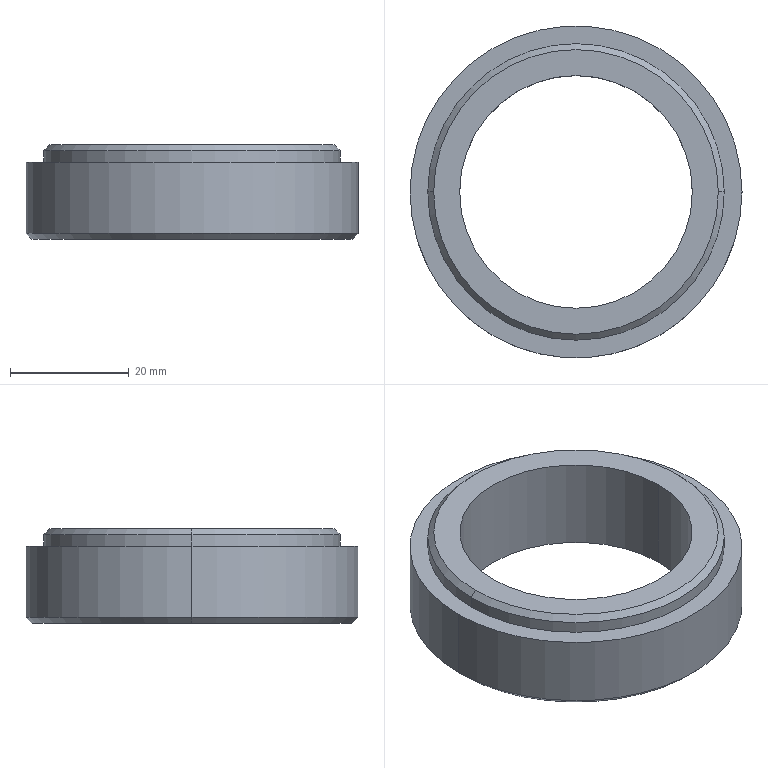Part | SolidWorks | features 3DProfileFeature 1, Chamfer 1, Extrusion 1, HoleWzd 1, ICE 1 | 1 solid | 13 faces | box 56 x 56 x 16 mm | volume 18386 mm3 | cylinder 6 | cone 4 | plane 3 | commonest cylinder face diameters 39.25 x2 50 x2 56 x2
STEP:
#1=CARTESIAN_POINT('',(-19.625,0.,0.));
#2=VERTEX_POINT('',#1);
#3=CARTESIAN_POINT('',(19.625,0.,0.));
#4=VERTEX_POINT('',#3);
#5=CARTESIAN_POINT('',(0.,0.,0.));
#6=DIRECTION('',(0.,0.,1.));
#7=DIRECTION('',(1.,0.,0.));
#8=AXIS2_PLACEMENT_3D('',#5,#6,#7);
#9=CIRCLE('',#8,19.625);
#10=EDGE_CURVE('',#2,#4,#9,.T.);
#11=ORIENTED_EDGE('',*,*,#10,.F.);
#12=CARTESIAN_POINT('',(-19.625,0.,16.));
#13=VERTEX_POINT('',#12);
#14=CARTESIAN_POINT('',(-19.625,0.,16.));
#15=DIRECTION('',(0.,0.,1.));
#16=VECTOR('',#15,1000.);
#17=LINE('',#14,#16);
#18=EDGE_CURVE('',#2,#13,#17,.T.);
#19=ORIENTED_EDGE('',*,*,#18,.T.);
#20=CARTESIAN_POINT('',(19.625,0.,16.));
#21=VERTEX_POINT('',#20);
#22=CARTESIAN_POINT('',(0.,0.,16.));
#23=DIRECTION('',(0.,0.,1.));
#24=DIRECTION('',(1.,0.,0.));
#25=AXIS2_PLACEMENT_3D('',#22,#23,#24);
#26=CIRCLE('',#25,19.625);
#27=EDGE_CURVE('',#13,#21,#26,.T.);
#28=ORIENTED_EDGE('',*,*,#27,.T.);
#29=CARTESIAN_POINT('',(19.625,0.,16.));
#30=DIRECTION('',(0.,0.,1.));
#31=VECTOR('',#30,1000.);
#32=LINE('',#29,#31);
#33=EDGE_CURVE('',#4,#21,#32,.T.);
#34=ORIENTED_EDGE('',*,*,#33,.F.);
#35=EDGE_LOOP('',(#11,#19,#28,#34));
#36=FACE_OUTER_BOUND('',#35,.T.);
#37=CARTESIAN_POINT('',(0.,0.,16.));
#38=DIRECTION('',(0.,0.,1.));
#39=DIRECTION('',(1.,0.,0.));
#40=AXIS2_PLACEMENT_3D('',#37,#38,#39);
#41=CYLINDRICAL_SURFACE('',#40,19.625);
#42=ADVANCED_FACE('',(#36),#41,.F.);
#43=CARTESIAN_POINT('',(24.,0.,16.));
#44=VERTEX_POINT('',#43);
#45=CARTESIAN_POINT('',(-24.,0.,16.));
#46=VERTEX_POINT('',#45);
#47=CARTESIAN_POINT('',(0.,0.,16.));
#48=DIRECTION('',(0.,0.,1.));
#49=DIRECTION('',(1.,0.,0.));
#50=AXIS2_PLACEMENT_3D('',#47,#48,#49);
#51=CIRCLE('',#50,24.);
#52=EDGE_CURVE('',#44,#46,#51,.T.);
#53=ORIENTED_EDGE('',*,*,#52,.F.);
#54=CARTESIAN_POINT('',(25.,0.,15.));
#55=VERTEX_POINT('',#54);
#56=CARTESIAN_POINT('',(24.,0.,16.));
#57=DIRECTION('',(0.7071,0.,-0.7071));
#58=VECTOR('',#57,1000.);
#59=LINE('',#56,#58);
#60=EDGE_CURVE('',#44,#55,#59,.T.);
#61=ORIENTED_EDGE('',*,*,#60,.T.);
#62=CARTESIAN_POINT('',(-25.,0.,15.));
#63=VERTEX_POINT('',#62);
#64=CARTESIAN_POINT('',(0.,0.,15.));
#65=DIRECTION('',(0.,0.,-1.));
#66=DIRECTION('',(1.,0.,0.));
#67=AXIS2_PLACEMENT_3D('',#64,#65,#66);
#68=CIRCLE('',#67,25.);
#69=EDGE_CURVE('',#63,#55,#68,.T.);
#70=ORIENTED_EDGE('',*,*,#69,.F.);
#71=CARTESIAN_POINT('',(-24.,0.,16.));
#72=DIRECTION('',(-0.7071,0.,-0.7071));
#73=VECTOR('',#72,1000.);
#74=LINE('',#71,#73);
#75=EDGE_CURVE('',#46,#63,#74,.T.);
#76=ORIENTED_EDGE('',*,*,#75,.F.);
#77=EDGE_LOOP('',(#53,#61,#70,#76));
#78=FACE_OUTER_BOUND('',#77,.T.);
#79=CARTESIAN_POINT('',(0.,0.,16.));
#80=DIRECTION('',(0.,0.,-1.));
#81=DIRECTION('',(-1.,0.,0.));
#82=AXIS2_PLACEMENT_3D('',#79,#80,#81);
#83=CONICAL_SURFACE('',#82,24.,0.7854);
#84=ADVANCED_FACE('',(#78),#83,.T.);
#85=CARTESIAN_POINT('',(-27.,0.,0.));
#86=VERTEX_POINT('',#85);
#87=CARTESIAN_POINT('',(27.,0.,0.));
#88=VERTEX_POINT('',#87);
#89=CARTESIAN_POINT('',(0.,0.,0.));
#90=DIRECTION('',(0.,0.,-1.));
#91=DIRECTION('',(1.,0.,0.));
#92=AXIS2_PLACEMENT_3D('',#89,#90,#91);
#93=CIRCLE('',#92,27.);
#94=EDGE_CURVE('',#86,#88,#93,.T.);
#95=ORIENTED_EDGE('',*,*,#94,.F.);
#96=CARTESIAN_POINT('',(-28.,0.,1.));
#97=VERTEX_POINT('',#96);
#98=CARTESIAN_POINT('',(-28.,0.,1.));
#99=DIRECTION('',(-0.7071,0.,0.7071));
#100=VECTOR('',#99,1000.);
#101=LINE('',#98,#100);
#102=EDGE_CURVE('',#86,#97,#101,.T.);
#103=ORIENTED_EDGE('',*,*,#102,.T.);
#104=CARTESIAN_POINT('',(28.,0.,1.));
#105=VERTEX_POINT('',#104);
#106=CARTESIAN_POINT('',(0.,0.,1.));
#107=DIRECTION('',(0.,0.,1.));
#108=DIRECTION('',(1.,0.,0.));
#109=AXIS2_PLACEMENT_3D('',#106,#107,#108);
#110=CIRCLE('',#109,28.);
#111=EDGE_CURVE('',#105,#97,#110,.T.);
#112=ORIENTED_EDGE('',*,*,#111,.F.);
#113=CARTESIAN_POINT('',(28.,0.,1.));
#114=DIRECTION('',(0.7071,0.,0.7071));
#115=VECTOR('',#114,1000.);
#116=LINE('',#113,#115);
#117=EDGE_CURVE('',#88,#105,#116,.T.);
#118=ORIENTED_EDGE('',*,*,#117,.F.);
#119=EDGE_LOOP('',(#95,#103,#112,#118));
#120=FACE_OUTER_BOUND('',#119,.T.);
#121=CARTESIAN_POINT('',(0.,0.,1.));
#122=DIRECTION('',(0.,0.,1.));
#123=DIRECTION('',(1.,0.,0.));
#124=AXIS2_PLACEMENT_3D('',#121,#122,#123);
#125=CONICAL_SURFACE('',#124,28.,0.7854);
#126=ADVANCED_FACE('',(#120),#125,.T.);
#127=ORIENTED_EDGE('',*,*,#69,.T.);
#128=CARTESIAN_POINT('',(25.,0.,13.));
#129=VERTEX_POINT('',#128);
#130=CARTESIAN_POINT('',(25.,0.,16.));
#131=DIRECTION('',(0.,0.,-1.));
#132=VECTOR('',#131,1000.);
#133=LINE('',#130,#132);
#134=EDGE_CURVE('',#55,#129,#133,.T.);
#135=ORIENTED_EDGE('',*,*,#134,.T.);
#136=CARTESIAN_POINT('',(-25.,0.,13.));
#137=VERTEX_POINT('',#136);
#138=CARTESIAN_POINT('',(0.,0.,13.));
#139=DIRECTION('',(0.,0.,1.));
#140=DIRECTION('',(1.,0.,0.));
#141=AXIS2_PLACEMENT_3D('',#138,#139,#140);
#142=CIRCLE('',#141,25.);
#143=EDGE_CURVE('',#129,#137,#142,.T.);
#144=ORIENTED_EDGE('',*,*,#143,.T.);
#145=CARTESIAN_POINT('',(-25.,0.,16.));
#146=DIRECTION('',(0.,0.,-1.));
#147=VECTOR('',#146,1000.);
#148=LINE('',#145,#147);
#149=EDGE_CURVE('',#63,#137,#148,.T.);
#150=ORIENTED_EDGE('',*,*,#149,.F.);
#151=EDGE_LOOP('',(#127,#135,#144,#150));
#152=FACE_OUTER_BOUND('',#151,.T.);
#153=CARTESIAN_POINT('',(0.,0.,16.));
#154=DIRECTION('',(0.,0.,-1.));
#155=DIRECTION('',(-1.,0.,0.));
#156=AXIS2_PLACEMENT_3D('',#153,#154,#155);
#157=CYLINDRICAL_SURFACE('',#156,25.);
#158=ADVANCED_FACE('',(#152),#157,.T.);
#159=CARTESIAN_POINT('',(28.,0.,13.));
#160=VERTEX_POINT('',#159);
#161=CARTESIAN_POINT('',(-28.,0.,13.));
#162=VERTEX_POINT('',#161);
#163=CARTESIAN_POINT('',(0.,0.,13.));
#164=DIRECTION('',(0.,0.,1.));
#165=DIRECTION('',(1.,0.,0.));
#166=AXIS2_PLACEMENT_3D('',#163,#164,#165);
#167=CIRCLE('',#166,28.);
#168=EDGE_CURVE('',#160,#162,#167,.T.);
#169=ORIENTED_EDGE('',*,*,#168,.F.);
#170=CARTESIAN_POINT('',(28.,0.,13.));
#171=DIRECTION('',(0.,0.,-1.));
#172=VECTOR('',#171,1000.);
#173=LINE('',#170,#172);
#174=EDGE_CURVE('',#160,#105,#173,.T.);
#175=ORIENTED_EDGE('',*,*,#174,.T.);
#176=ORIENTED_EDGE('',*,*,#111,.T.);
#177=CARTESIAN_POINT('',(-28.,0.,13.));
#178=DIRECTION('',(0.,0.,-1.));
#179=VECTOR('',#178,1000.);
#180=LINE('',#177,#179);
#181=EDGE_CURVE('',#162,#97,#180,.T.);
#182=ORIENTED_EDGE('',*,*,#181,.F.);
#183=EDGE_LOOP('',(#169,#175,#176,#182));
#184=FACE_OUTER_BOUND('',#183,.T.);
#185=CARTESIAN_POINT('',(0.,0.,13.));
#186=DIRECTION('',(0.,0.,-1.));
#187=DIRECTION('',(-1.,0.,0.));
#188=AXIS2_PLACEMENT_3D('',#185,#186,#187);
#189=CYLINDRICAL_SURFACE('',#188,28.);
#190=ADVANCED_FACE('',(#184),#189,.T.);
#191=CARTESIAN_POINT('',(0.,0.,13.));
#192=DIRECTION('',(0.,0.,1.));
#193=DIRECTION('',(1.,0.,0.));
#194=AXIS2_PLACEMENT_3D('',#191,#192,#193);
#195=CIRCLE('',#194,28.);
#196=EDGE_CURVE('',#162,#160,#195,.T.);
#197=ORIENTED_EDGE('',*,*,#196,.T.);
#198=ORIENTED_EDGE('',*,*,#168,.T.);
#199=EDGE_LOOP('',(#197,#198));
#200=FACE_OUTER_BOUND('',#199,.T.);
#201=CARTESIAN_POINT('',(0.,0.,13.));
#202=DIRECTION('',(0.,0.,1.));
#203=DIRECTION('',(1.,0.,0.));
#204=AXIS2_PLACEMENT_3D('',#201,#202,#203);
#205=CIRCLE('',#204,25.);
#206=EDGE_CURVE('',#137,#129,#205,.T.);
#207=ORIENTED_EDGE('',*,*,#206,.F.);
#208=ORIENTED_EDGE('',*,*,#143,.F.);
#209=EDGE_LOOP('',(#207,#208));
#210=FACE_BOUND('',#209,.T.);
#211=CARTESIAN_POINT('',(0.,0.,13.));
#212=DIRECTION('',(0.,0.,1.));
#213=DIRECTION('',(1.,0.,0.));
#214=AXIS2_PLACEMENT_3D('',#211,#212,#213);
#215=PLANE('',#214);
#216=ADVANCED_FACE('',(#200,#210),#215,.T.);
#217=ORIENTED_EDGE('',*,*,#174,.F.);
#218=ORIENTED_EDGE('',*,*,#196,.F.);
#219=ORIENTED_EDGE('',*,*,#181,.T.);
#220=CARTESIAN_POINT('',(0.,0.,1.));
#221=DIRECTION('',(0.,0.,1.));
#222=DIRECTION('',(1.,0.,0.));
#223=AXIS2_PLACEMENT_3D('',#220,#221,#222);
#224=CIRCLE('',#223,28.);
#225=EDGE_CURVE('',#97,#105,#224,.T.);
#226=ORIENTED_EDGE('',*,*,#225,.T.);
#227=EDGE_LOOP('',(#217,#218,#219,#226));
#228=FACE_OUTER_BOUND('',#227,.T.);
#229=CARTESIAN_POINT('',(0.,0.,13.));
#230=DIRECTION('',(0.,0.,-1.));
#231=DIRECTION('',(-1.,0.,0.));
#232=AXIS2_PLACEMENT_3D('',#229,#230,#231);
#233=CYLINDRICAL_SURFACE('',#232,28.);
#234=ADVANCED_FACE('',(#228),#233,.T.);
#235=CARTESIAN_POINT('',(0.,0.,0.));
#236=DIRECTION('',(0.,0.,1.));
#237=DIRECTION('',(1.,0.,0.));
#238=AXIS2_PLACEMENT_3D('',#235,#236,#237);
#239=CIRCLE('',#238,19.625);
#240=EDGE_CURVE('',#4,#2,#239,.T.);
#241=ORIENTED_EDGE('',*,*,#240,.T.);
#242=ORIENTED_EDGE('',*,*,#10,.T.);
#243=EDGE_LOOP('',(#241,#242));
#244=FACE_BOUND('',#243,.T.);
#245=CARTESIAN_POINT('',(0.,0.,0.));
#246=DIRECTION('',(0.,0.,-1.));
#247=DIRECTION('',(1.,0.,0.));
#248=AXIS2_PLACEMENT_3D('',#245,#246,#247);
#249=CIRCLE('',#248,27.);
#250=EDGE_CURVE('',#88,#86,#249,.T.);
#251=ORIENTED_EDGE('',*,*,#250,.T.);
#252=ORIENTED_EDGE('',*,*,#94,.T.);
#253=EDGE_LOOP('',(#251,#252));
#254=FACE_OUTER_BOUND('',#253,.T.);
#255=CARTESIAN_POINT('',(0.,0.,0.));
#256=DIRECTION('',(0.,0.,1.));
#257=DIRECTION('',(1.,0.,0.));
#258=AXIS2_PLACEMENT_3D('',#255,#256,#257);
#259=PLANE('',#258);
#260=ADVANCED_FACE('',(#244,#254),#259,.F.);
#261=ORIENTED_EDGE('',*,*,#134,.F.);
#262=CARTESIAN_POINT('',(0.,0.,15.));
#263=DIRECTION('',(0.,0.,-1.));
#264=DIRECTION('',(1.,0.,0.));
#265=AXIS2_PLACEMENT_3D('',#262,#263,#264);
#266=CIRCLE('',#265,25.);
#267=EDGE_CURVE('',#55,#63,#266,.T.);
#268=ORIENTED_EDGE('',*,*,#267,.T.);
#269=ORIENTED_EDGE('',*,*,#149,.T.);
#270=ORIENTED_EDGE('',*,*,#206,.T.);
#271=EDGE_LOOP('',(#261,#268,#269,#270));
#272=FACE_OUTER_BOUND('',#271,.T.);
#273=CARTESIAN_POINT('',(0.,0.,16.));
#274=DIRECTION('',(0.,0.,-1.));
#275=DIRECTION('',(-1.,0.,0.));
#276=AXIS2_PLACEMENT_3D('',#273,#274,#275);
#277=CYLINDRICAL_SURFACE('',#276,25.);
#278=ADVANCED_FACE('',(#272),#277,.T.);
#279=CARTESIAN_POINT('',(0.,0.,16.));
#280=DIRECTION('',(0.,0.,1.));
#281=DIRECTION('',(1.,0.,0.));
#282=AXIS2_PLACEMENT_3D('',#279,#280,#281);
#283=CIRCLE('',#282,19.625);
#284=EDGE_CURVE('',#21,#13,#283,.T.);
#285=ORIENTED_EDGE('',*,*,#284,.F.);
#286=ORIENTED_EDGE('',*,*,#27,.F.);
#287=EDGE_LOOP('',(#285,#286));
#288=FACE_BOUND('',#287,.T.);
#289=CARTESIAN_POINT('',(0.,0.,16.));
#290=DIRECTION('',(0.,0.,1.));
#291=DIRECTION('',(1.,0.,0.));
#292=AXIS2_PLACEMENT_3D('',#289,#290,#291);
#293=CIRCLE('',#292,24.);
#294=EDGE_CURVE('',#46,#44,#293,.T.);
#295=ORIENTED_EDGE('',*,*,#294,.T.);
#296=ORIENTED_EDGE('',*,*,#52,.T.);
#297=EDGE_LOOP('',(#295,#296));
#298=FACE_OUTER_BOUND('',#297,.T.);
#299=CARTESIAN_POINT('',(0.,0.,16.));
#300=DIRECTION('',(0.,0.,1.));
#301=DIRECTION('',(1.,0.,0.));
#302=AXIS2_PLACEMENT_3D('',#299,#300,#301);
#303=PLANE('',#302);
#304=ADVANCED_FACE('',(#288,#298),#303,.T.);
#305=ORIENTED_EDGE('',*,*,#102,.F.);
#306=ORIENTED_EDGE('',*,*,#250,.F.);
#307=ORIENTED_EDGE('',*,*,#117,.T.);
#308=ORIENTED_EDGE('',*,*,#225,.F.);
#309=EDGE_LOOP('',(#305,#306,#307,#308));
#310=FACE_OUTER_BOUND('',#309,.T.);
#311=CARTESIAN_POINT('',(0.,0.,1.));
#312=DIRECTION('',(0.,0.,1.));
#313=DIRECTION('',(1.,0.,0.));
#314=AXIS2_PLACEMENT_3D('',#311,#312,#313);
#315=CONICAL_SURFACE('',#314,28.,0.7854);
#316=ADVANCED_FACE('',(#310),#315,.T.);
#317=ORIENTED_EDGE('',*,*,#60,.F.);
#318=ORIENTED_EDGE('',*,*,#294,.F.);
#319=ORIENTED_EDGE('',*,*,#75,.T.);
#320=ORIENTED_EDGE('',*,*,#267,.F.);
#321=EDGE_LOOP('',(#317,#318,#319,#320));
#322=FACE_OUTER_BOUND('',#321,.T.);
#323=CARTESIAN_POINT('',(0.,0.,16.));
#324=DIRECTION('',(0.,0.,-1.));
#325=DIRECTION('',(-1.,0.,0.));
#326=AXIS2_PLACEMENT_3D('',#323,#324,#325);
#327=CONICAL_SURFACE('',#326,24.,0.7854);
#328=ADVANCED_FACE('',(#322),#327,.T.);
#329=ORIENTED_EDGE('',*,*,#18,.F.);
#330=ORIENTED_EDGE('',*,*,#240,.F.);
#331=ORIENTED_EDGE('',*,*,#33,.T.);
#332=ORIENTED_EDGE('',*,*,#284,.T.);
#333=EDGE_LOOP('',(#329,#330,#331,#332));
#334=FACE_OUTER_BOUND('',#333,.T.);
#335=CARTESIAN_POINT('',(0.,0.,16.));
#336=DIRECTION('',(0.,0.,1.));
#337=DIRECTION('',(1.,0.,0.));
#338=AXIS2_PLACEMENT_3D('',#335,#336,#337);
#339=CYLINDRICAL_SURFACE('',#338,19.625);
#340=ADVANCED_FACE('',(#334),#339,.F.);
#341=CLOSED_SHELL('',(#42,#84,#126,#158,#190,#216,#234,#260,#278,#304,#316,#328,#340));
#342=MANIFOLD_SOLID_BREP('',#341);
#343=CARTESIAN_POINT('',(0.,0.,0.));
#344=DIRECTION('',(0.,0.,1.));
#345=DIRECTION('',(1.,0.,0.));
#346=AXIS2_PLACEMENT_3D('',#343,#344,#345);
#347=(LENGTH_UNIT()NAMED_UNIT(*)SI_UNIT(.MILLI.,.METRE.));
#348=UNCERTAINTY_MEASURE_WITH_UNIT(LENGTH_MEASURE(0.00001),#347,'','');
#349=(NAMED_UNIT(*)PLANE_ANGLE_UNIT()SI_UNIT($,.RADIAN.));
#350=(NAMED_UNIT(*)SI_UNIT($,.STERADIAN.)SOLID_ANGLE_UNIT());
#351=(GEOMETRIC_REPRESENTATION_CONTEXT(3)GLOBAL_UNCERTAINTY_ASSIGNED_CONTEXT((#348))GLOBAL_UNIT_ASSIGNED_CONTEXT((#347,#349,#350))REPRESENTATION_CONTEXT('',''));
#352=ADVANCED_BREP_SHAPE_REPRESENTATION('',(#342,#346),#351);